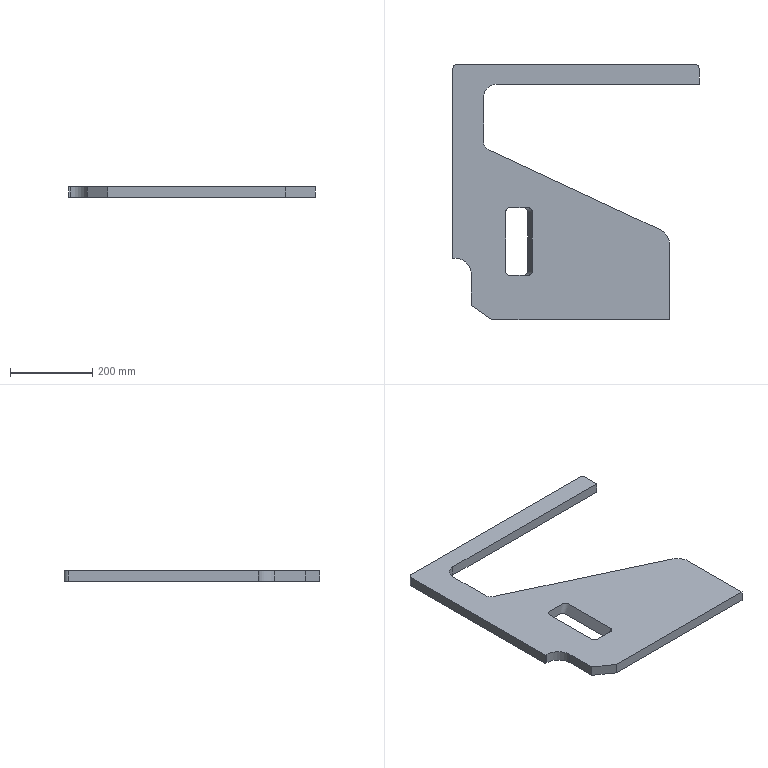Part | SolidWorks | features BlendCut 1, Extrusion 1 | 1 solid | 21 faces | box 600 x 622.5 x 25 mm | volume 4943914 mm3 | plane 13 | cylinder 6 | spline 2 | commonest cylinder face diameters 20 x2 80 x2 40 x1 60 x1
STEP:
#1=CARTESIAN_POINT('',(182.5,263.,0.));
#2=VERTEX_POINT('',#1);
#3=CARTESIAN_POINT('',(182.5,118.,0.));
#4=VERTEX_POINT('',#3);
#5=CARTESIAN_POINT('',(182.5,263.,0.));
#6=DIRECTION('',(0.,-1.,0.));
#7=VECTOR('',#6,1000.);
#8=LINE('',#5,#7);
#9=EDGE_CURVE('',#2,#4,#8,.T.);
#10=ORIENTED_EDGE('',*,*,#9,.T.);
#11=CARTESIAN_POINT('',(193.5,118.,25.));
#12=VERTEX_POINT('',#11);
#13=CARTESIAN_POINT('',(182.5,118.,0.));
#14=CARTESIAN_POINT('',(193.5,118.,25.));
#15=B_SPLINE_CURVE_WITH_KNOTS('',1,(#13,#14),.UNSPECIFIED.,.F.,.F.,(2,2),(0.,1.),.UNSPECIFIED.);
#16=EDGE_CURVE('',#4,#12,#15,.T.);
#17=ORIENTED_EDGE('',*,*,#16,.T.);
#18=CARTESIAN_POINT('',(193.5,263.,25.));
#19=VERTEX_POINT('',#18);
#20=CARTESIAN_POINT('',(193.5,263.,25.));
#21=DIRECTION('',(0.,1.,0.));
#22=VECTOR('',#21,1000.);
#23=LINE('',#20,#22);
#24=EDGE_CURVE('',#12,#19,#23,.T.);
#25=ORIENTED_EDGE('',*,*,#24,.T.);
#26=CARTESIAN_POINT('',(183.5,273.,25.));
#27=VERTEX_POINT('',#26);
#28=CARTESIAN_POINT('',(183.5,263.,25.));
#29=DIRECTION('',(0.,0.,1.));
#30=DIRECTION('',(-1.,0.,0.));
#31=AXIS2_PLACEMENT_3D('',#28,#29,#30);
#32=CIRCLE('',#31,10.);
#33=EDGE_CURVE('',#19,#27,#32,.T.);
#34=ORIENTED_EDGE('',*,*,#33,.T.);
#35=CARTESIAN_POINT('',(138.5,273.,25.));
#36=VERTEX_POINT('',#35);
#37=CARTESIAN_POINT('',(138.5,273.,25.));
#38=DIRECTION('',(-1.,0.,0.));
#39=VECTOR('',#38,1000.);
#40=LINE('',#37,#39);
#41=EDGE_CURVE('',#27,#36,#40,.T.);
#42=ORIENTED_EDGE('',*,*,#41,.T.);
#43=CARTESIAN_POINT('',(128.5,263.,25.));
#44=VERTEX_POINT('',#43);
#45=CARTESIAN_POINT('',(138.5,263.,25.));
#46=DIRECTION('',(0.,0.,1.));
#47=DIRECTION('',(-1.,0.,0.));
#48=AXIS2_PLACEMENT_3D('',#45,#46,#47);
#49=CIRCLE('',#48,10.);
#50=EDGE_CURVE('',#36,#44,#49,.T.);
#51=ORIENTED_EDGE('',*,*,#50,.T.);
#52=CARTESIAN_POINT('',(128.5,263.,0.));
#53=VERTEX_POINT('',#52);
#54=CARTESIAN_POINT('',(128.5,263.,0.));
#55=CARTESIAN_POINT('',(128.5,263.,25.));
#56=B_SPLINE_CURVE_WITH_KNOTS('',1,(#54,#55),.UNSPECIFIED.,.F.,.F.,(2,2),(0.,1.),.UNSPECIFIED.);
#57=EDGE_CURVE('',#53,#44,#56,.T.);
#58=ORIENTED_EDGE('',*,*,#57,.F.);
#59=CARTESIAN_POINT('',(138.5,273.,0.));
#60=VERTEX_POINT('',#59);
#61=CARTESIAN_POINT('',(138.5,263.,0.));
#62=DIRECTION('',(0.,0.,-1.));
#63=DIRECTION('',(-1.,0.,0.));
#64=AXIS2_PLACEMENT_3D('',#61,#62,#63);
#65=CIRCLE('',#64,10.);
#66=EDGE_CURVE('',#53,#60,#65,.T.);
#67=ORIENTED_EDGE('',*,*,#66,.T.);
#68=CARTESIAN_POINT('',(172.5,273.,0.));
#69=VERTEX_POINT('',#68);
#70=CARTESIAN_POINT('',(138.5,273.,0.));
#71=DIRECTION('',(1.,0.,0.));
#72=VECTOR('',#71,1000.);
#73=LINE('',#70,#72);
#74=EDGE_CURVE('',#60,#69,#73,.T.);
#75=ORIENTED_EDGE('',*,*,#74,.T.);
#76=CARTESIAN_POINT('',(172.5,263.,0.));
#77=DIRECTION('',(0.,0.,-1.));
#78=DIRECTION('',(1.,0.,0.));
#79=AXIS2_PLACEMENT_3D('',#76,#77,#78);
#80=CIRCLE('',#79,10.);
#81=EDGE_CURVE('',#69,#2,#80,.T.);
#82=ORIENTED_EDGE('',*,*,#81,.T.);
#83=EDGE_LOOP('',(#10,#17,#25,#34,#42,#51,#58,#67,#75,#82));
#84=FACE_OUTER_BOUND('',#83,.T.);
#85=CARTESIAN_POINT('',(128.5,263.,0.));
#86=CARTESIAN_POINT('',(128.5,263.,25.));
#87=CARTESIAN_POINT('',(128.5,250.917,0.));
#88=CARTESIAN_POINT('',(128.5,250.917,25.));
#89=CARTESIAN_POINT('',(128.5,226.75,0.));
#90=CARTESIAN_POINT('',(128.5,226.75,25.));
#91=CARTESIAN_POINT('',(128.5,190.5,0.));
#92=CARTESIAN_POINT('',(128.5,190.5,25.));
#93=CARTESIAN_POINT('',(128.5,154.25,0.));
#94=CARTESIAN_POINT('',(128.5,154.25,25.));
#95=CARTESIAN_POINT('',(128.5,130.083,0.));
#96=CARTESIAN_POINT('',(128.5,130.083,25.));
#97=CARTESIAN_POINT('',(128.5,116.691,0.));
#98=CARTESIAN_POINT('',(128.5,116.691,25.));
#99=CARTESIAN_POINT('',(129.027,113.997,0.));
#100=CARTESIAN_POINT('',(129.014,114.136,25.));
#101=CARTESIAN_POINT('',(131.408,110.559,0.));
#102=CARTESIAN_POINT('',(131.118,110.896,25.));
#103=CARTESIAN_POINT('',(134.844,108.424,0.));
#104=CARTESIAN_POINT('',(134.338,108.618,25.));
#105=CARTESIAN_POINT('',(137.318,108.,0.));
#106=CARTESIAN_POINT('',(137.057,108.,25.));
#107=CARTESIAN_POINT('',(141.461,108.,0.));
#108=CARTESIAN_POINT('',(142.116,108.,25.));
#109=CARTESIAN_POINT('',(147.179,108.,0.));
#110=CARTESIAN_POINT('',(149.538,108.,25.));
#111=CARTESIAN_POINT('',(155.5,108.,0.));
#112=CARTESIAN_POINT('',(161.,108.,25.));
#113=CARTESIAN_POINT('',(163.821,108.,0.));
#114=CARTESIAN_POINT('',(172.462,108.,25.));
#115=CARTESIAN_POINT('',(169.539,108.,0.));
#116=CARTESIAN_POINT('',(179.884,108.,25.));
#117=CARTESIAN_POINT('',(173.682,108.,0.));
#118=CARTESIAN_POINT('',(184.943,108.,25.));
#119=CARTESIAN_POINT('',(176.156,108.424,0.));
#120=CARTESIAN_POINT('',(187.662,108.618,25.));
#121=CARTESIAN_POINT('',(179.592,110.559,0.));
#122=CARTESIAN_POINT('',(190.882,110.896,25.));
#123=CARTESIAN_POINT('',(181.973,113.997,0.));
#124=CARTESIAN_POINT('',(192.986,114.136,25.));
#125=CARTESIAN_POINT('',(182.5,116.691,0.));
#126=CARTESIAN_POINT('',(193.5,116.691,25.));
#127=CARTESIAN_POINT('',(182.5,130.083,0.));
#128=CARTESIAN_POINT('',(193.5,130.083,25.));
#129=CARTESIAN_POINT('',(182.5,154.25,0.));
#130=CARTESIAN_POINT('',(193.5,154.25,25.));
#131=CARTESIAN_POINT('',(182.5,190.5,0.));
#132=CARTESIAN_POINT('',(193.5,190.5,25.));
#133=CARTESIAN_POINT('',(182.5,226.75,0.));
#134=CARTESIAN_POINT('',(193.5,226.75,25.));
#135=CARTESIAN_POINT('',(182.5,250.917,0.));
#136=CARTESIAN_POINT('',(193.5,250.917,25.));
#137=CARTESIAN_POINT('',(182.5,264.309,0.));
#138=CARTESIAN_POINT('',(193.5,264.309,25.));
#139=CARTESIAN_POINT('',(181.973,267.003,0.));
#140=CARTESIAN_POINT('',(192.986,266.864,25.));
#141=CARTESIAN_POINT('',(179.592,270.441,0.));
#142=CARTESIAN_POINT('',(190.882,270.104,25.));
#143=CARTESIAN_POINT('',(176.156,272.576,0.));
#144=CARTESIAN_POINT('',(187.662,272.382,25.));
#145=CARTESIAN_POINT('',(173.682,273.,0.));
#146=CARTESIAN_POINT('',(184.943,273.,25.));
#147=CARTESIAN_POINT('',(169.539,273.,0.));
#148=CARTESIAN_POINT('',(179.884,273.,25.));
#149=CARTESIAN_POINT('',(163.821,273.,0.));
#150=CARTESIAN_POINT('',(172.462,273.,25.));
#151=CARTESIAN_POINT('',(155.5,273.,0.));
#152=CARTESIAN_POINT('',(161.,273.,25.));
#153=CARTESIAN_POINT('',(147.179,273.,0.));
#154=CARTESIAN_POINT('',(149.538,273.,25.));
#155=CARTESIAN_POINT('',(141.461,273.,0.));
#156=CARTESIAN_POINT('',(142.116,273.,25.));
#157=CARTESIAN_POINT('',(137.318,273.,0.));
#158=CARTESIAN_POINT('',(137.057,273.,25.));
#159=CARTESIAN_POINT('',(134.844,272.576,0.));
#160=CARTESIAN_POINT('',(134.338,272.382,25.));
#161=CARTESIAN_POINT('',(131.408,270.441,0.));
#162=CARTESIAN_POINT('',(131.118,270.104,25.));
#163=CARTESIAN_POINT('',(129.027,267.003,0.));
#164=CARTESIAN_POINT('',(129.014,266.864,25.));
#165=CARTESIAN_POINT('',(128.5,264.309,0.));
#166=CARTESIAN_POINT('',(128.5,264.309,25.));
#167=CARTESIAN_POINT('',(128.5,263.,0.));
#168=CARTESIAN_POINT('',(128.5,263.,25.));
#169=B_SPLINE_SURFACE_WITH_KNOTS('',3,1,((#85,#86),(#87,#88),(#89,#90),(#91,#92),(#93,#94),(#95,#96),(#97,#98),(#99,#100),(#101,#102),(#103,#104),(#105,#106),(#107,#108),(#109,#110),(#111,#112),(#113,#114),(#115,#116),(#117,#118),(#119,#120),(#121,#122),(#123,#124),(#125,#126),(#127,#128),(#129,#130),(#131,#132),(#133,#134),(#135,#136),(#137,#138),(#139,#140),(#141,#142),(#143,#144),(#145,#146),(#147,#148),(#149,#150),(#151,#152),(#153,#154),(#155,#156),(#157,#158),(#159,#160),(#161,#162),(#163,#164),(#165,#166),(#167,#168)),.UNSPECIFIED.,.T.,.F.,.F.,(4,1,1,1,2,1,1,1,2,1,1,1,2,1,1,1,2,1,1,1,2,1,1,1,2,1,1,1,2,1,1,1,4),(2,2),(0.,0.084,0.168,0.252,0.336,0.3451,0.3542,0.3633,0.3724,0.3952,0.418,0.4408,0.4636,0.4727,0.4818,0.4909,0.5,0.584,0.668,0.752,0.836,0.8451,0.8542,0.8633,0.8724,0.8952,0.918,0.9408,0.9636,0.9727,0.9818,0.9909,1.),(0.,1.),.UNSPECIFIED.);
#170=ADVANCED_FACE('',(#84),#169,.F.);
#171=CARTESIAN_POINT('',(5.,150.,0.));
#172=VERTEX_POINT('',#171);
#173=CARTESIAN_POINT('',(45.,110.,0.));
#174=VERTEX_POINT('',#173);
#175=CARTESIAN_POINT('',(5.,110.,0.));
#176=DIRECTION('',(0.,0.,-1.));
#177=DIRECTION('',(-1.,0.,0.));
#178=AXIS2_PLACEMENT_3D('',#175,#176,#177);
#179=CIRCLE('',#178,40.);
#180=EDGE_CURVE('',#172,#174,#179,.T.);
#181=ORIENTED_EDGE('',*,*,#180,.T.);
#182=CARTESIAN_POINT('',(45.,110.,25.));
#183=VERTEX_POINT('',#182);
#184=CARTESIAN_POINT('',(45.,110.,25.));
#185=DIRECTION('',(0.,0.,-1.));
#186=VECTOR('',#185,1000.);
#187=LINE('',#184,#186);
#188=EDGE_CURVE('',#183,#174,#187,.T.);
#189=ORIENTED_EDGE('',*,*,#188,.F.);
#190=CARTESIAN_POINT('',(5.,150.,25.));
#191=VERTEX_POINT('',#190);
#192=CARTESIAN_POINT('',(5.,110.,25.));
#193=DIRECTION('',(0.,0.,-1.));
#194=DIRECTION('',(-1.,0.,0.));
#195=AXIS2_PLACEMENT_3D('',#192,#193,#194);
#196=CIRCLE('',#195,40.);
#197=EDGE_CURVE('',#191,#183,#196,.T.);
#198=ORIENTED_EDGE('',*,*,#197,.F.);
#199=CARTESIAN_POINT('',(5.,150.,25.));
#200=DIRECTION('',(0.,0.,-1.));
#201=VECTOR('',#200,1000.);
#202=LINE('',#199,#201);
#203=EDGE_CURVE('',#191,#172,#202,.T.);
#204=ORIENTED_EDGE('',*,*,#203,.T.);
#205=EDGE_LOOP('',(#181,#189,#198,#204));
#206=FACE_OUTER_BOUND('',#205,.T.);
#207=CARTESIAN_POINT('',(5.,110.,25.));
#208=DIRECTION('',(0.,0.,-1.));
#209=DIRECTION('',(-1.,0.,0.));
#210=AXIS2_PLACEMENT_3D('',#207,#208,#209);
#211=CYLINDRICAL_SURFACE('',#210,40.);
#212=ADVANCED_FACE('',(#206),#211,.F.);
#213=CARTESIAN_POINT('',(45.,35.01,0.));
#214=VERTEX_POINT('',#213);
#215=CARTESIAN_POINT('',(45.,35.01,0.));
#216=DIRECTION('',(0.,-1.,0.));
#217=VECTOR('',#216,1000.);
#218=LINE('',#215,#217);
#219=EDGE_CURVE('',#174,#214,#218,.T.);
#220=ORIENTED_EDGE('',*,*,#219,.T.);
#221=CARTESIAN_POINT('',(45.,35.01,25.));
#222=VERTEX_POINT('',#221);
#223=CARTESIAN_POINT('',(45.,35.01,25.));
#224=DIRECTION('',(0.,0.,-1.));
#225=VECTOR('',#224,1000.);
#226=LINE('',#223,#225);
#227=EDGE_CURVE('',#222,#214,#226,.T.);
#228=ORIENTED_EDGE('',*,*,#227,.F.);
#229=CARTESIAN_POINT('',(45.,35.01,25.));
#230=DIRECTION('',(0.,-1.,0.));
#231=VECTOR('',#230,1000.);
#232=LINE('',#229,#231);
#233=EDGE_CURVE('',#183,#222,#232,.T.);
#234=ORIENTED_EDGE('',*,*,#233,.F.);
#235=ORIENTED_EDGE('',*,*,#188,.T.);
#236=EDGE_LOOP('',(#220,#228,#234,#235));
#237=FACE_OUTER_BOUND('',#236,.T.);
#238=CARTESIAN_POINT('',(45.,35.01,25.));
#239=DIRECTION('',(1.,0.,0.));
#240=DIRECTION('',(0.,0.,-1.));
#241=AXIS2_PLACEMENT_3D('',#238,#239,#240);
#242=PLANE('',#241);
#243=ADVANCED_FACE('',(#237),#242,.F.);
#244=CARTESIAN_POINT('',(95.,0.,0.));
#245=VERTEX_POINT('',#244);
#246=CARTESIAN_POINT('',(95.,0.,0.));
#247=DIRECTION('',(0.8192,-0.5736,0.));
#248=VECTOR('',#247,1000.);
#249=LINE('',#246,#248);
#250=EDGE_CURVE('',#214,#245,#249,.T.);
#251=ORIENTED_EDGE('',*,*,#250,.T.);
#252=CARTESIAN_POINT('',(95.,0.,25.));
#253=VERTEX_POINT('',#252);
#254=CARTESIAN_POINT('',(95.,0.,25.));
#255=DIRECTION('',(0.,0.,-1.));
#256=VECTOR('',#255,1000.);
#257=LINE('',#254,#256);
#258=EDGE_CURVE('',#253,#245,#257,.T.);
#259=ORIENTED_EDGE('',*,*,#258,.F.);
#260=CARTESIAN_POINT('',(95.,0.,25.));
#261=DIRECTION('',(0.8192,-0.5736,0.));
#262=VECTOR('',#261,1000.);
#263=LINE('',#260,#262);
#264=EDGE_CURVE('',#222,#253,#263,.T.);
#265=ORIENTED_EDGE('',*,*,#264,.F.);
#266=ORIENTED_EDGE('',*,*,#227,.T.);
#267=EDGE_LOOP('',(#251,#259,#265,#266));
#268=FACE_OUTER_BOUND('',#267,.T.);
#269=CARTESIAN_POINT('',(95.,0.,25.));
#270=DIRECTION('',(0.5736,0.8192,0.));
#271=DIRECTION('',(-0.8192,0.5736,0.));
#272=AXIS2_PLACEMENT_3D('',#269,#270,#271);
#273=PLANE('',#272);
#274=ADVANCED_FACE('',(#268),#273,.F.);
#275=CARTESIAN_POINT('',(528.,0.,0.));
#276=VERTEX_POINT('',#275);
#277=CARTESIAN_POINT('',(528.,0.,0.));
#278=DIRECTION('',(1.,0.,0.));
#279=VECTOR('',#278,1000.);
#280=LINE('',#277,#279);
#281=EDGE_CURVE('',#245,#276,#280,.T.);
#282=ORIENTED_EDGE('',*,*,#281,.T.);
#283=CARTESIAN_POINT('',(528.,0.,25.));
#284=VERTEX_POINT('',#283);
#285=CARTESIAN_POINT('',(528.,0.,25.));
#286=DIRECTION('',(0.,0.,-1.));
#287=VECTOR('',#286,1000.);
#288=LINE('',#285,#287);
#289=EDGE_CURVE('',#284,#276,#288,.T.);
#290=ORIENTED_EDGE('',*,*,#289,.F.);
#291=CARTESIAN_POINT('',(528.,0.,25.));
#292=DIRECTION('',(1.,0.,0.));
#293=VECTOR('',#292,1000.);
#294=LINE('',#291,#293);
#295=EDGE_CURVE('',#253,#284,#294,.T.);
#296=ORIENTED_EDGE('',*,*,#295,.F.);
#297=ORIENTED_EDGE('',*,*,#258,.T.);
#298=EDGE_LOOP('',(#282,#290,#296,#297));
#299=FACE_OUTER_BOUND('',#298,.T.);
#300=CARTESIAN_POINT('',(528.,0.,25.));
#301=DIRECTION('',(0.,1.,0.));
#302=DIRECTION('',(-1.,0.,0.));
#303=AXIS2_PLACEMENT_3D('',#300,#301,#302);
#304=PLANE('',#303);
#305=ADVANCED_FACE('',(#299),#304,.F.);
#306=CARTESIAN_POINT('',(528.,183.025,0.));
#307=VERTEX_POINT('',#306);
#308=CARTESIAN_POINT('',(528.,183.025,0.));
#309=DIRECTION('',(0.,1.,0.));
#310=VECTOR('',#309,1000.);
#311=LINE('',#308,#310);
#312=EDGE_CURVE('',#276,#307,#311,.T.);
#313=ORIENTED_EDGE('',*,*,#312,.T.);
#314=CARTESIAN_POINT('',(528.,183.025,25.));
#315=VERTEX_POINT('',#314);
#316=CARTESIAN_POINT('',(528.,183.025,25.));
#317=DIRECTION('',(0.,0.,-1.));
#318=VECTOR('',#317,1000.);
#319=LINE('',#316,#318);
#320=EDGE_CURVE('',#315,#307,#319,.T.);
#321=ORIENTED_EDGE('',*,*,#320,.F.);
#322=CARTESIAN_POINT('',(528.,183.025,25.));
#323=DIRECTION('',(0.,1.,0.));
#324=VECTOR('',#323,1000.);
#325=LINE('',#322,#324);
#326=EDGE_CURVE('',#284,#315,#325,.T.);
#327=ORIENTED_EDGE('',*,*,#326,.F.);
#328=ORIENTED_EDGE('',*,*,#289,.T.);
#329=EDGE_LOOP('',(#313,#321,#327,#328));
#330=FACE_OUTER_BOUND('',#329,.T.);
#331=CARTESIAN_POINT('',(528.,183.025,25.));
#332=DIRECTION('',(-1.,0.,0.));
#333=DIRECTION('',(0.,0.,1.));
#334=AXIS2_PLACEMENT_3D('',#331,#332,#333);
#335=PLANE('',#334);
#336=ADVANCED_FACE('',(#330),#335,.F.);
#337=CARTESIAN_POINT('',(504.915,219.273,0.));
#338=VERTEX_POINT('',#337);
#339=CARTESIAN_POINT('',(488.,183.025,0.));
#340=DIRECTION('',(0.,0.,1.));
#341=DIRECTION('',(1.,0.,0.));
#342=AXIS2_PLACEMENT_3D('',#339,#340,#341);
#343=CIRCLE('',#342,40.);
#344=EDGE_CURVE('',#307,#338,#343,.T.);
#345=ORIENTED_EDGE('',*,*,#344,.T.);
#346=CARTESIAN_POINT('',(504.915,219.273,25.));
#347=VERTEX_POINT('',#346);
#348=CARTESIAN_POINT('',(504.915,219.273,25.));
#349=DIRECTION('',(0.,0.,-1.));
#350=VECTOR('',#349,1000.);
#351=LINE('',#348,#350);
#352=EDGE_CURVE('',#347,#338,#351,.T.);
#353=ORIENTED_EDGE('',*,*,#352,.F.);
#354=CARTESIAN_POINT('',(488.,183.025,25.));
#355=DIRECTION('',(0.,0.,1.));
#356=DIRECTION('',(1.,0.,0.));
#357=AXIS2_PLACEMENT_3D('',#354,#355,#356);
#358=CIRCLE('',#357,40.);
#359=EDGE_CURVE('',#315,#347,#358,.T.);
#360=ORIENTED_EDGE('',*,*,#359,.F.);
#361=ORIENTED_EDGE('',*,*,#320,.T.);
#362=EDGE_LOOP('',(#345,#353,#360,#361));
#363=FACE_OUTER_BOUND('',#362,.T.);
#364=CARTESIAN_POINT('',(488.,183.025,25.));
#365=DIRECTION('',(0.,0.,-1.));
#366=DIRECTION('',(-1.,0.,0.));
#367=AXIS2_PLACEMENT_3D('',#364,#365,#366);
#368=CYLINDRICAL_SURFACE('',#367,40.);
#369=ADVANCED_FACE('',(#363),#368,.T.);
#370=CARTESIAN_POINT('',(86.542,414.514,0.));
#371=VERTEX_POINT('',#370);
#372=CARTESIAN_POINT('',(86.542,414.514,0.));
#373=DIRECTION('',(-0.9062,0.4229,0.));
#374=VECTOR('',#373,1000.);
#375=LINE('',#372,#374);
#376=EDGE_CURVE('',#338,#371,#375,.T.);
#377=ORIENTED_EDGE('',*,*,#376,.T.);
#378=CARTESIAN_POINT('',(86.542,414.514,25.));
#379=VERTEX_POINT('',#378);
#380=CARTESIAN_POINT('',(86.542,414.514,25.));
#381=DIRECTION('',(0.,0.,-1.));
#382=VECTOR('',#381,1000.);
#383=LINE('',#380,#382);
#384=EDGE_CURVE('',#379,#371,#383,.T.);
#385=ORIENTED_EDGE('',*,*,#384,.F.);
#386=CARTESIAN_POINT('',(86.542,414.514,25.));
#387=DIRECTION('',(-0.9062,0.4229,0.));
#388=VECTOR('',#387,1000.);
#389=LINE('',#386,#388);
#390=EDGE_CURVE('',#347,#379,#389,.T.);
#391=ORIENTED_EDGE('',*,*,#390,.F.);
#392=ORIENTED_EDGE('',*,*,#352,.T.);
#393=EDGE_LOOP('',(#377,#385,#391,#392));
#394=FACE_OUTER_BOUND('',#393,.T.);
#395=CARTESIAN_POINT('',(86.542,414.514,25.));
#396=DIRECTION('',(-0.4229,-0.9062,0.));
#397=DIRECTION('',(0.9062,-0.4229,0.));
#398=AXIS2_PLACEMENT_3D('',#395,#396,#397);
#399=PLANE('',#398);
#400=ADVANCED_FACE('',(#394),#399,.F.);
#401=CARTESIAN_POINT('',(75.,432.637,0.));
#402=VERTEX_POINT('',#401);
#403=CARTESIAN_POINT('',(95.,432.637,0.));
#404=DIRECTION('',(0.,0.,-1.));
#405=DIRECTION('',(1.,0.,0.));
#406=AXIS2_PLACEMENT_3D('',#403,#404,#405);
#407=CIRCLE('',#406,20.);
#408=EDGE_CURVE('',#371,#402,#407,.T.);
#409=ORIENTED_EDGE('',*,*,#408,.T.);
#410=CARTESIAN_POINT('',(75.,432.637,25.));
#411=VERTEX_POINT('',#410);
#412=CARTESIAN_POINT('',(75.,432.637,25.));
#413=DIRECTION('',(0.,0.,-1.));
#414=VECTOR('',#413,1000.);
#415=LINE('',#412,#414);
#416=EDGE_CURVE('',#411,#402,#415,.T.);
#417=ORIENTED_EDGE('',*,*,#416,.F.);
#418=CARTESIAN_POINT('',(95.,432.637,25.));
#419=DIRECTION('',(0.,0.,-1.));
#420=DIRECTION('',(1.,0.,0.));
#421=AXIS2_PLACEMENT_3D('',#418,#419,#420);
#422=CIRCLE('',#421,20.);
#423=EDGE_CURVE('',#379,#411,#422,.T.);
#424=ORIENTED_EDGE('',*,*,#423,.F.);
#425=ORIENTED_EDGE('',*,*,#384,.T.);
#426=EDGE_LOOP('',(#409,#417,#424,#425));
#427=FACE_OUTER_BOUND('',#426,.T.);
#428=CARTESIAN_POINT('',(95.,432.637,25.));
#429=DIRECTION('',(0.,0.,-1.));
#430=DIRECTION('',(-1.,0.,0.));
#431=AXIS2_PLACEMENT_3D('',#428,#429,#430);
#432=CYLINDRICAL_SURFACE('',#431,20.);
#433=ADVANCED_FACE('',(#427),#432,.F.);
#434=CARTESIAN_POINT('',(75.,543.5,0.));
#435=VERTEX_POINT('',#434);
#436=CARTESIAN_POINT('',(75.,543.5,0.));
#437=DIRECTION('',(0.,1.,0.));
#438=VECTOR('',#437,1000.);
#439=LINE('',#436,#438);
#440=EDGE_CURVE('',#402,#435,#439,.T.);
#441=ORIENTED_EDGE('',*,*,#440,.T.);
#442=CARTESIAN_POINT('',(75.,543.5,25.));
#443=VERTEX_POINT('',#442);
#444=CARTESIAN_POINT('',(75.,543.5,25.));
#445=DIRECTION('',(0.,0.,-1.));
#446=VECTOR('',#445,1000.);
#447=LINE('',#444,#446);
#448=EDGE_CURVE('',#443,#435,#447,.T.);
#449=ORIENTED_EDGE('',*,*,#448,.F.);
#450=CARTESIAN_POINT('',(75.,543.5,25.));
#451=DIRECTION('',(0.,1.,0.));
#452=VECTOR('',#451,1000.);
#453=LINE('',#450,#452);
#454=EDGE_CURVE('',#411,#443,#453,.T.);
#455=ORIENTED_EDGE('',*,*,#454,.F.);
#456=ORIENTED_EDGE('',*,*,#416,.T.);
#457=EDGE_LOOP('',(#441,#449,#455,#456));
#458=FACE_OUTER_BOUND('',#457,.T.);
#459=CARTESIAN_POINT('',(75.,543.5,25.));
#460=DIRECTION('',(-1.,0.,0.));
#461=DIRECTION('',(0.,-1.,0.));
#462=AXIS2_PLACEMENT_3D('',#459,#460,#461);
#463=PLANE('',#462);
#464=ADVANCED_FACE('',(#458),#463,.F.);
#465=CARTESIAN_POINT('',(105.,573.5,0.));
#466=VERTEX_POINT('',#465);
#467=CARTESIAN_POINT('',(105.,543.5,0.));
#468=DIRECTION('',(0.,0.,-1.));
#469=DIRECTION('',(-1.,0.,0.));
#470=AXIS2_PLACEMENT_3D('',#467,#468,#469);
#471=CIRCLE('',#470,30.);
#472=EDGE_CURVE('',#435,#466,#471,.T.);
#473=ORIENTED_EDGE('',*,*,#472,.T.);
#474=CARTESIAN_POINT('',(105.,573.5,25.));
#475=VERTEX_POINT('',#474);
#476=CARTESIAN_POINT('',(105.,573.5,25.));
#477=DIRECTION('',(0.,0.,-1.));
#478=VECTOR('',#477,1000.);
#479=LINE('',#476,#478);
#480=EDGE_CURVE('',#475,#466,#479,.T.);
#481=ORIENTED_EDGE('',*,*,#480,.F.);
#482=CARTESIAN_POINT('',(105.,543.5,25.));
#483=DIRECTION('',(0.,0.,-1.));
#484=DIRECTION('',(-1.,0.,0.));
#485=AXIS2_PLACEMENT_3D('',#482,#483,#484);
#486=CIRCLE('',#485,30.);
#487=EDGE_CURVE('',#443,#475,#486,.T.);
#488=ORIENTED_EDGE('',*,*,#487,.F.);
#489=ORIENTED_EDGE('',*,*,#448,.T.);
#490=EDGE_LOOP('',(#473,#481,#488,#489));
#491=FACE_OUTER_BOUND('',#490,.T.);
#492=CARTESIAN_POINT('',(105.,543.5,25.));
#493=DIRECTION('',(0.,0.,-1.));
#494=DIRECTION('',(-1.,0.,0.));
#495=AXIS2_PLACEMENT_3D('',#492,#493,#494);
#496=CYLINDRICAL_SURFACE('',#495,30.);
#497=ADVANCED_FACE('',(#491),#496,.F.);
#498=CARTESIAN_POINT('',(600.,573.5,0.));
#499=VERTEX_POINT('',#498);
#500=CARTESIAN_POINT('',(600.,573.5,0.));
#501=DIRECTION('',(1.,0.,0.));
#502=VECTOR('',#501,1000.);
#503=LINE('',#500,#502);
#504=EDGE_CURVE('',#466,#499,#503,.T.);
#505=ORIENTED_EDGE('',*,*,#504,.T.);
#506=CARTESIAN_POINT('',(600.,573.5,25.));
#507=VERTEX_POINT('',#506);
#508=CARTESIAN_POINT('',(600.,573.5,25.));
#509=DIRECTION('',(0.,0.,-1.));
#510=VECTOR('',#509,1000.);
#511=LINE('',#508,#510);
#512=EDGE_CURVE('',#507,#499,#511,.T.);
#513=ORIENTED_EDGE('',*,*,#512,.F.);
#514=CARTESIAN_POINT('',(600.,573.5,25.));
#515=DIRECTION('',(1.,0.,0.));
#516=VECTOR('',#515,1000.);
#517=LINE('',#514,#516);
#518=EDGE_CURVE('',#475,#507,#517,.T.);
#519=ORIENTED_EDGE('',*,*,#518,.F.);
#520=ORIENTED_EDGE('',*,*,#480,.T.);
#521=EDGE_LOOP('',(#505,#513,#519,#520));
#522=FACE_OUTER_BOUND('',#521,.T.);
#523=CARTESIAN_POINT('',(600.,573.5,25.));
#524=DIRECTION('',(0.,1.,0.));
#525=DIRECTION('',(-1.,0.,0.));
#526=AXIS2_PLACEMENT_3D('',#523,#524,#525);
#527=PLANE('',#526);
#528=ADVANCED_FACE('',(#522),#527,.F.);
#529=CARTESIAN_POINT('',(600.,612.5,0.));
#530=VERTEX_POINT('',#529);
#531=CARTESIAN_POINT('',(600.,612.5,0.));
#532=DIRECTION('',(0.,1.,0.));
#533=VECTOR('',#532,1000.);
#534=LINE('',#531,#533);
#535=EDGE_CURVE('',#499,#530,#534,.T.);
#536=ORIENTED_EDGE('',*,*,#535,.T.);
#537=CARTESIAN_POINT('',(600.,612.5,25.));
#538=VERTEX_POINT('',#537);
#539=CARTESIAN_POINT('',(600.,612.5,25.));
#540=DIRECTION('',(0.,0.,-1.));
#541=VECTOR('',#540,1000.);
#542=LINE('',#539,#541);
#543=EDGE_CURVE('',#538,#530,#542,.T.);
#544=ORIENTED_EDGE('',*,*,#543,.F.);
#545=CARTESIAN_POINT('',(600.,612.5,25.));
#546=DIRECTION('',(0.,1.,0.));
#547=VECTOR('',#546,1000.);
#548=LINE('',#545,#547);
#549=EDGE_CURVE('',#507,#538,#548,.T.);
#550=ORIENTED_EDGE('',*,*,#549,.F.);
#551=ORIENTED_EDGE('',*,*,#512,.T.);
#552=EDGE_LOOP('',(#536,#544,#550,#551));
#553=FACE_OUTER_BOUND('',#552,.T.);
#554=CARTESIAN_POINT('',(600.,612.5,25.));
#555=DIRECTION('',(-1.,0.,0.));
#556=DIRECTION('',(0.,0.,1.));
#557=AXIS2_PLACEMENT_3D('',#554,#555,#556);
#558=PLANE('',#557);
#559=ADVANCED_FACE('',(#553),#558,.F.);
#560=CARTESIAN_POINT('',(590.,622.5,0.));
#561=VERTEX_POINT('',#560);
#562=CARTESIAN_POINT('',(590.,612.5,0.));
#563=DIRECTION('',(0.,0.,1.));
#564=DIRECTION('',(-1.,0.,0.));
#565=AXIS2_PLACEMENT_3D('',#562,#563,#564);
#566=CIRCLE('',#565,10.);
#567=EDGE_CURVE('',#530,#561,#566,.T.);
#568=ORIENTED_EDGE('',*,*,#567,.T.);
#569=CARTESIAN_POINT('',(590.,622.5,25.));
#570=VERTEX_POINT('',#569);
#571=CARTESIAN_POINT('',(590.,622.5,25.));
#572=DIRECTION('',(0.,0.,-1.));
#573=VECTOR('',#572,1000.);
#574=LINE('',#571,#573);
#575=EDGE_CURVE('',#570,#561,#574,.T.);
#576=ORIENTED_EDGE('',*,*,#575,.F.);
#577=CARTESIAN_POINT('',(590.,612.5,25.));
#578=DIRECTION('',(0.,0.,1.));
#579=DIRECTION('',(-1.,0.,0.));
#580=AXIS2_PLACEMENT_3D('',#577,#578,#579);
#581=CIRCLE('',#580,10.);
#582=EDGE_CURVE('',#538,#570,#581,.T.);
#583=ORIENTED_EDGE('',*,*,#582,.F.);
#584=ORIENTED_EDGE('',*,*,#543,.T.);
#585=EDGE_LOOP('',(#568,#576,#583,#584));
#586=FACE_OUTER_BOUND('',#585,.T.);
#587=CARTESIAN_POINT('',(590.,612.5,25.));
#588=DIRECTION('',(0.,0.,-1.));
#589=DIRECTION('',(-1.,0.,0.));
#590=AXIS2_PLACEMENT_3D('',#587,#588,#589);
#591=CYLINDRICAL_SURFACE('',#590,10.);
#592=ADVANCED_FACE('',(#586),#591,.T.);
#593=CARTESIAN_POINT('',(10.,622.5,0.));
#594=VERTEX_POINT('',#593);
#595=CARTESIAN_POINT('',(10.,622.5,0.));
#596=DIRECTION('',(-1.,0.,0.));
#597=VECTOR('',#596,1000.);
#598=LINE('',#595,#597);
#599=EDGE_CURVE('',#561,#594,#598,.T.);
#600=ORIENTED_EDGE('',*,*,#599,.T.);
#601=CARTESIAN_POINT('',(10.,622.5,25.));
#602=VERTEX_POINT('',#601);
#603=CARTESIAN_POINT('',(10.,622.5,25.));
#604=DIRECTION('',(0.,0.,-1.));
#605=VECTOR('',#604,1000.);
#606=LINE('',#603,#605);
#607=EDGE_CURVE('',#602,#594,#606,.T.);
#608=ORIENTED_EDGE('',*,*,#607,.F.);
#609=CARTESIAN_POINT('',(10.,622.5,25.));
#610=DIRECTION('',(-1.,0.,0.));
#611=VECTOR('',#610,1000.);
#612=LINE('',#609,#611);
#613=EDGE_CURVE('',#570,#602,#612,.T.);
#614=ORIENTED_EDGE('',*,*,#613,.F.);
#615=ORIENTED_EDGE('',*,*,#575,.T.);
#616=EDGE_LOOP('',(#600,#608,#614,#615));
#617=FACE_OUTER_BOUND('',#616,.T.);
#618=CARTESIAN_POINT('',(10.,622.5,25.));
#619=DIRECTION('',(0.,-1.,0.));
#620=DIRECTION('',(0.,0.,-1.));
#621=AXIS2_PLACEMENT_3D('',#618,#619,#620);
#622=PLANE('',#621);
#623=ADVANCED_FACE('',(#617),#622,.F.);
#624=CARTESIAN_POINT('',(0.,612.5,0.));
#625=VERTEX_POINT('',#624);
#626=CARTESIAN_POINT('',(10.,612.5,0.));
#627=DIRECTION('',(0.,0.,1.));
#628=DIRECTION('',(-1.,0.,0.));
#629=AXIS2_PLACEMENT_3D('',#626,#627,#628);
#630=CIRCLE('',#629,10.);
#631=EDGE_CURVE('',#594,#625,#630,.T.);
#632=ORIENTED_EDGE('',*,*,#631,.T.);
#633=CARTESIAN_POINT('',(0.,612.5,25.));
#634=VERTEX_POINT('',#633);
#635=CARTESIAN_POINT('',(0.,612.5,25.));
#636=DIRECTION('',(0.,0.,-1.));
#637=VECTOR('',#636,1000.);
#638=LINE('',#635,#637);
#639=EDGE_CURVE('',#634,#625,#638,.T.);
#640=ORIENTED_EDGE('',*,*,#639,.F.);
#641=CARTESIAN_POINT('',(10.,612.5,25.));
#642=DIRECTION('',(0.,0.,1.));
#643=DIRECTION('',(-1.,0.,0.));
#644=AXIS2_PLACEMENT_3D('',#641,#642,#643);
#645=CIRCLE('',#644,10.);
#646=EDGE_CURVE('',#602,#634,#645,.T.);
#647=ORIENTED_EDGE('',*,*,#646,.F.);
#648=ORIENTED_EDGE('',*,*,#607,.T.);
#649=EDGE_LOOP('',(#632,#640,#647,#648));
#650=FACE_OUTER_BOUND('',#649,.T.);
#651=CARTESIAN_POINT('',(10.,612.5,25.));
#652=DIRECTION('',(0.,0.,-1.));
#653=DIRECTION('',(-1.,0.,0.));
#654=AXIS2_PLACEMENT_3D('',#651,#652,#653);
#655=CYLINDRICAL_SURFACE('',#654,10.);
#656=ADVANCED_FACE('',(#650),#655,.T.);
#657=CARTESIAN_POINT('',(0.,150.,0.));
#658=VERTEX_POINT('',#657);
#659=CARTESIAN_POINT('',(0.,150.,0.));
#660=DIRECTION('',(0.,-1.,0.));
#661=VECTOR('',#660,1000.);
#662=LINE('',#659,#661);
#663=EDGE_CURVE('',#625,#658,#662,.T.);
#664=ORIENTED_EDGE('',*,*,#663,.T.);
#665=CARTESIAN_POINT('',(0.,150.,25.));
#666=VERTEX_POINT('',#665);
#667=CARTESIAN_POINT('',(0.,150.,25.));
#668=DIRECTION('',(0.,0.,-1.));
#669=VECTOR('',#668,1000.);
#670=LINE('',#667,#669);
#671=EDGE_CURVE('',#666,#658,#670,.T.);
#672=ORIENTED_EDGE('',*,*,#671,.F.);
#673=CARTESIAN_POINT('',(0.,150.,25.));
#674=DIRECTION('',(0.,-1.,0.));
#675=VECTOR('',#674,1000.);
#676=LINE('',#673,#675);
#677=EDGE_CURVE('',#634,#666,#676,.T.);
#678=ORIENTED_EDGE('',*,*,#677,.F.);
#679=ORIENTED_EDGE('',*,*,#639,.T.);
#680=EDGE_LOOP('',(#664,#672,#678,#679));
#681=FACE_OUTER_BOUND('',#680,.T.);
#682=CARTESIAN_POINT('',(0.,150.,25.));
#683=DIRECTION('',(1.,0.,0.));
#684=DIRECTION('',(0.,0.,-1.));
#685=AXIS2_PLACEMENT_3D('',#682,#683,#684);
#686=PLANE('',#685);
#687=ADVANCED_FACE('',(#681),#686,.F.);
#688=CARTESIAN_POINT('',(5.,150.,0.));
#689=DIRECTION('',(1.,0.,0.));
#690=VECTOR('',#689,1000.);
#691=LINE('',#688,#690);
#692=EDGE_CURVE('',#658,#172,#691,.T.);
#693=ORIENTED_EDGE('',*,*,#692,.T.);
#694=ORIENTED_EDGE('',*,*,#203,.F.);
#695=CARTESIAN_POINT('',(5.,150.,25.));
#696=DIRECTION('',(1.,0.,0.));
#697=VECTOR('',#696,1000.);
#698=LINE('',#695,#697);
#699=EDGE_CURVE('',#666,#191,#698,.T.);
#700=ORIENTED_EDGE('',*,*,#699,.F.);
#701=ORIENTED_EDGE('',*,*,#671,.T.);
#702=EDGE_LOOP('',(#693,#694,#700,#701));
#703=FACE_OUTER_BOUND('',#702,.T.);
#704=CARTESIAN_POINT('',(5.,150.,25.));
#705=DIRECTION('',(0.,1.,0.));
#706=DIRECTION('',(0.,0.,1.));
#707=AXIS2_PLACEMENT_3D('',#704,#705,#706);
#708=PLANE('',#707);
#709=ADVANCED_FACE('',(#703),#708,.F.);
#710=CARTESIAN_POINT('',(128.5,118.,25.));
#711=VERTEX_POINT('',#710);
#712=CARTESIAN_POINT('',(128.5,263.,25.));
#713=DIRECTION('',(0.,-1.,0.));
#714=VECTOR('',#713,1000.);
#715=LINE('',#712,#714);
#716=EDGE_CURVE('',#44,#711,#715,.T.);
#717=ORIENTED_EDGE('',*,*,#716,.F.);
#718=ORIENTED_EDGE('',*,*,#50,.F.);
#719=ORIENTED_EDGE('',*,*,#41,.F.);
#720=ORIENTED_EDGE('',*,*,#33,.F.);
#721=ORIENTED_EDGE('',*,*,#24,.F.);
#722=CARTESIAN_POINT('',(183.5,108.,25.));
#723=VERTEX_POINT('',#722);
#724=CARTESIAN_POINT('',(183.5,118.,25.));
#725=DIRECTION('',(0.,0.,1.));
#726=DIRECTION('',(-1.,0.,0.));
#727=AXIS2_PLACEMENT_3D('',#724,#725,#726);
#728=CIRCLE('',#727,10.);
#729=EDGE_CURVE('',#723,#12,#728,.T.);
#730=ORIENTED_EDGE('',*,*,#729,.F.);
#731=CARTESIAN_POINT('',(138.5,108.,25.));
#732=VERTEX_POINT('',#731);
#733=CARTESIAN_POINT('',(138.5,108.,25.));
#734=DIRECTION('',(1.,0.,0.));
#735=VECTOR('',#734,1000.);
#736=LINE('',#733,#735);
#737=EDGE_CURVE('',#732,#723,#736,.T.);
#738=ORIENTED_EDGE('',*,*,#737,.F.);
#739=CARTESIAN_POINT('',(138.5,118.,25.));
#740=DIRECTION('',(0.,0.,1.));
#741=DIRECTION('',(1.,0.,0.));
#742=AXIS2_PLACEMENT_3D('',#739,#740,#741);
#743=CIRCLE('',#742,10.);
#744=EDGE_CURVE('',#711,#732,#743,.T.);
#745=ORIENTED_EDGE('',*,*,#744,.F.);
#746=EDGE_LOOP('',(#717,#718,#719,#720,#721,#730,#738,#745));
#747=FACE_BOUND('',#746,.T.);
#748=ORIENTED_EDGE('',*,*,#197,.T.);
#749=ORIENTED_EDGE('',*,*,#233,.T.);
#750=ORIENTED_EDGE('',*,*,#264,.T.);
#751=ORIENTED_EDGE('',*,*,#295,.T.);
#752=ORIENTED_EDGE('',*,*,#326,.T.);
#753=ORIENTED_EDGE('',*,*,#359,.T.);
#754=ORIENTED_EDGE('',*,*,#390,.T.);
#755=ORIENTED_EDGE('',*,*,#423,.T.);
#756=ORIENTED_EDGE('',*,*,#454,.T.);
#757=ORIENTED_EDGE('',*,*,#487,.T.);
#758=ORIENTED_EDGE('',*,*,#518,.T.);
#759=ORIENTED_EDGE('',*,*,#549,.T.);
#760=ORIENTED_EDGE('',*,*,#582,.T.);
#761=ORIENTED_EDGE('',*,*,#613,.T.);
#762=ORIENTED_EDGE('',*,*,#646,.T.);
#763=ORIENTED_EDGE('',*,*,#677,.T.);
#764=ORIENTED_EDGE('',*,*,#699,.T.);
#765=EDGE_LOOP('',(#748,#749,#750,#751,#752,#753,#754,#755,#756,#757,#758,#759,#760,#761,#762,#763,#764));
#766=FACE_OUTER_BOUND('',#765,.T.);
#767=CARTESIAN_POINT('',(5.,110.,25.));
#768=DIRECTION('',(0.,0.,-1.));
#769=DIRECTION('',(-1.,0.,0.));
#770=AXIS2_PLACEMENT_3D('',#767,#768,#769);
#771=PLANE('',#770);
#772=ADVANCED_FACE('',(#747,#766),#771,.F.);
#773=ORIENTED_EDGE('',*,*,#66,.F.);
#774=CARTESIAN_POINT('',(128.5,118.,0.));
#775=VERTEX_POINT('',#774);
#776=CARTESIAN_POINT('',(128.5,263.,0.));
#777=DIRECTION('',(0.,1.,0.));
#778=VECTOR('',#777,1000.);
#779=LINE('',#776,#778);
#780=EDGE_CURVE('',#775,#53,#779,.T.);
#781=ORIENTED_EDGE('',*,*,#780,.F.);
#782=CARTESIAN_POINT('',(138.5,108.,0.));
#783=VERTEX_POINT('',#782);
#784=CARTESIAN_POINT('',(138.5,118.,0.));
#785=DIRECTION('',(0.,0.,-1.));
#786=DIRECTION('',(-1.,0.,0.));
#787=AXIS2_PLACEMENT_3D('',#784,#785,#786);
#788=CIRCLE('',#787,10.);
#789=EDGE_CURVE('',#783,#775,#788,.T.);
#790=ORIENTED_EDGE('',*,*,#789,.F.);
#791=CARTESIAN_POINT('',(172.5,108.,0.));
#792=VERTEX_POINT('',#791);
#793=CARTESIAN_POINT('',(138.5,108.,0.));
#794=DIRECTION('',(-1.,0.,0.));
#795=VECTOR('',#794,1000.);
#796=LINE('',#793,#795);
#797=EDGE_CURVE('',#792,#783,#796,.T.);
#798=ORIENTED_EDGE('',*,*,#797,.F.);
#799=CARTESIAN_POINT('',(172.5,118.,0.));
#800=DIRECTION('',(0.,0.,-1.));
#801=DIRECTION('',(1.,0.,0.));
#802=AXIS2_PLACEMENT_3D('',#799,#800,#801);
#803=CIRCLE('',#802,10.);
#804=EDGE_CURVE('',#4,#792,#803,.T.);
#805=ORIENTED_EDGE('',*,*,#804,.F.);
#806=ORIENTED_EDGE('',*,*,#9,.F.);
#807=ORIENTED_EDGE('',*,*,#81,.F.);
#808=ORIENTED_EDGE('',*,*,#74,.F.);
#809=EDGE_LOOP('',(#773,#781,#790,#798,#805,#806,#807,#808));
#810=FACE_BOUND('',#809,.T.);
#811=ORIENTED_EDGE('',*,*,#180,.F.);
#812=ORIENTED_EDGE('',*,*,#692,.F.);
#813=ORIENTED_EDGE('',*,*,#663,.F.);
#814=ORIENTED_EDGE('',*,*,#631,.F.);
#815=ORIENTED_EDGE('',*,*,#599,.F.);
#816=ORIENTED_EDGE('',*,*,#567,.F.);
#817=ORIENTED_EDGE('',*,*,#535,.F.);
#818=ORIENTED_EDGE('',*,*,#504,.F.);
#819=ORIENTED_EDGE('',*,*,#472,.F.);
#820=ORIENTED_EDGE('',*,*,#440,.F.);
#821=ORIENTED_EDGE('',*,*,#408,.F.);
#822=ORIENTED_EDGE('',*,*,#376,.F.);
#823=ORIENTED_EDGE('',*,*,#344,.F.);
#824=ORIENTED_EDGE('',*,*,#312,.F.);
#825=ORIENTED_EDGE('',*,*,#281,.F.);
#826=ORIENTED_EDGE('',*,*,#250,.F.);
#827=ORIENTED_EDGE('',*,*,#219,.F.);
#828=EDGE_LOOP('',(#811,#812,#813,#814,#815,#816,#817,#818,#819,#820,#821,#822,#823,#824,#825,#826,#827));
#829=FACE_OUTER_BOUND('',#828,.T.);
#830=CARTESIAN_POINT('',(5.,110.,0.));
#831=DIRECTION('',(0.,0.,-1.));
#832=DIRECTION('',(-1.,0.,0.));
#833=AXIS2_PLACEMENT_3D('',#830,#831,#832);
#834=PLANE('',#833);
#835=ADVANCED_FACE('',(#810,#829),#834,.T.);
#836=ORIENTED_EDGE('',*,*,#16,.F.);
#837=ORIENTED_EDGE('',*,*,#804,.T.);
#838=ORIENTED_EDGE('',*,*,#797,.T.);
#839=ORIENTED_EDGE('',*,*,#789,.T.);
#840=ORIENTED_EDGE('',*,*,#780,.T.);
#841=ORIENTED_EDGE('',*,*,#57,.T.);
#842=ORIENTED_EDGE('',*,*,#716,.T.);
#843=ORIENTED_EDGE('',*,*,#744,.T.);
#844=ORIENTED_EDGE('',*,*,#737,.T.);
#845=ORIENTED_EDGE('',*,*,#729,.T.);
#846=EDGE_LOOP('',(#836,#837,#838,#839,#840,#841,#842,#843,#844,#845));
#847=FACE_OUTER_BOUND('',#846,.T.);
#848=CARTESIAN_POINT('',(128.5,263.,0.));
#849=CARTESIAN_POINT('',(128.5,263.,25.));
#850=CARTESIAN_POINT('',(128.5,250.917,0.));
#851=CARTESIAN_POINT('',(128.5,250.917,25.));
#852=CARTESIAN_POINT('',(128.5,226.75,0.));
#853=CARTESIAN_POINT('',(128.5,226.75,25.));
#854=CARTESIAN_POINT('',(128.5,190.5,0.));
#855=CARTESIAN_POINT('',(128.5,190.5,25.));
#856=CARTESIAN_POINT('',(128.5,154.25,0.));
#857=CARTESIAN_POINT('',(128.5,154.25,25.));
#858=CARTESIAN_POINT('',(128.5,130.083,0.));
#859=CARTESIAN_POINT('',(128.5,130.083,25.));
#860=CARTESIAN_POINT('',(128.5,116.691,0.));
#861=CARTESIAN_POINT('',(128.5,116.691,25.));
#862=CARTESIAN_POINT('',(129.027,113.997,0.));
#863=CARTESIAN_POINT('',(129.014,114.136,25.));
#864=CARTESIAN_POINT('',(131.408,110.559,0.));
#865=CARTESIAN_POINT('',(131.118,110.896,25.));
#866=CARTESIAN_POINT('',(134.844,108.424,0.));
#867=CARTESIAN_POINT('',(134.338,108.618,25.));
#868=CARTESIAN_POINT('',(137.318,108.,0.));
#869=CARTESIAN_POINT('',(137.057,108.,25.));
#870=CARTESIAN_POINT('',(141.461,108.,0.));
#871=CARTESIAN_POINT('',(142.116,108.,25.));
#872=CARTESIAN_POINT('',(147.179,108.,0.));
#873=CARTESIAN_POINT('',(149.538,108.,25.));
#874=CARTESIAN_POINT('',(155.5,108.,0.));
#875=CARTESIAN_POINT('',(161.,108.,25.));
#876=CARTESIAN_POINT('',(163.821,108.,0.));
#877=CARTESIAN_POINT('',(172.462,108.,25.));
#878=CARTESIAN_POINT('',(169.539,108.,0.));
#879=CARTESIAN_POINT('',(179.884,108.,25.));
#880=CARTESIAN_POINT('',(173.682,108.,0.));
#881=CARTESIAN_POINT('',(184.943,108.,25.));
#882=CARTESIAN_POINT('',(176.156,108.424,0.));
#883=CARTESIAN_POINT('',(187.662,108.618,25.));
#884=CARTESIAN_POINT('',(179.592,110.559,0.));
#885=CARTESIAN_POINT('',(190.882,110.896,25.));
#886=CARTESIAN_POINT('',(181.973,113.997,0.));
#887=CARTESIAN_POINT('',(192.986,114.136,25.));
#888=CARTESIAN_POINT('',(182.5,116.691,0.));
#889=CARTESIAN_POINT('',(193.5,116.691,25.));
#890=CARTESIAN_POINT('',(182.5,130.083,0.));
#891=CARTESIAN_POINT('',(193.5,130.083,25.));
#892=CARTESIAN_POINT('',(182.5,154.25,0.));
#893=CARTESIAN_POINT('',(193.5,154.25,25.));
#894=CARTESIAN_POINT('',(182.5,190.5,0.));
#895=CARTESIAN_POINT('',(193.5,190.5,25.));
#896=CARTESIAN_POINT('',(182.5,226.75,0.));
#897=CARTESIAN_POINT('',(193.5,226.75,25.));
#898=CARTESIAN_POINT('',(182.5,250.917,0.));
#899=CARTESIAN_POINT('',(193.5,250.917,25.));
#900=CARTESIAN_POINT('',(182.5,264.309,0.));
#901=CARTESIAN_POINT('',(193.5,264.309,25.));
#902=CARTESIAN_POINT('',(181.973,267.003,0.));
#903=CARTESIAN_POINT('',(192.986,266.864,25.));
#904=CARTESIAN_POINT('',(179.592,270.441,0.));
#905=CARTESIAN_POINT('',(190.882,270.104,25.));
#906=CARTESIAN_POINT('',(176.156,272.576,0.));
#907=CARTESIAN_POINT('',(187.662,272.382,25.));
#908=CARTESIAN_POINT('',(173.682,273.,0.));
#909=CARTESIAN_POINT('',(184.943,273.,25.));
#910=CARTESIAN_POINT('',(169.539,273.,0.));
#911=CARTESIAN_POINT('',(179.884,273.,25.));
#912=CARTESIAN_POINT('',(163.821,273.,0.));
#913=CARTESIAN_POINT('',(172.462,273.,25.));
#914=CARTESIAN_POINT('',(155.5,273.,0.));
#915=CARTESIAN_POINT('',(161.,273.,25.));
#916=CARTESIAN_POINT('',(147.179,273.,0.));
#917=CARTESIAN_POINT('',(149.538,273.,25.));
#918=CARTESIAN_POINT('',(141.461,273.,0.));
#919=CARTESIAN_POINT('',(142.116,273.,25.));
#920=CARTESIAN_POINT('',(137.318,273.,0.));
#921=CARTESIAN_POINT('',(137.057,273.,25.));
#922=CARTESIAN_POINT('',(134.844,272.576,0.));
#923=CARTESIAN_POINT('',(134.338,272.382,25.));
#924=CARTESIAN_POINT('',(131.408,270.441,0.));
#925=CARTESIAN_POINT('',(131.118,270.104,25.));
#926=CARTESIAN_POINT('',(129.027,267.003,0.));
#927=CARTESIAN_POINT('',(129.014,266.864,25.));
#928=CARTESIAN_POINT('',(128.5,264.309,0.));
#929=CARTESIAN_POINT('',(128.5,264.309,25.));
#930=CARTESIAN_POINT('',(128.5,263.,0.));
#931=CARTESIAN_POINT('',(128.5,263.,25.));
#932=B_SPLINE_SURFACE_WITH_KNOTS('',3,1,((#848,#849),(#850,#851),(#852,#853),(#854,#855),(#856,#857),(#858,#859),(#860,#861),(#862,#863),(#864,#865),(#866,#867),(#868,#869),(#870,#871),(#872,#873),(#874,#875),(#876,#877),(#878,#879),(#880,#881),(#882,#883),(#884,#885),(#886,#887),(#888,#889),(#890,#891),(#892,#893),(#894,#895),(#896,#897),(#898,#899),(#900,#901),(#902,#903),(#904,#905),(#906,#907),(#908,#909),(#910,#911),(#912,#913),(#914,#915),(#916,#917),(#918,#919),(#920,#921),(#922,#923),(#924,#925),(#926,#927),(#928,#929),(#930,#931)),.UNSPECIFIED.,.T.,.F.,.F.,(4,1,1,1,2,1,1,1,2,1,1,1,2,1,1,1,2,1,1,1,2,1,1,1,2,1,1,1,2,1,1,1,4),(2,2),(0.,0.084,0.168,0.252,0.336,0.3451,0.3542,0.3633,0.3724,0.3952,0.418,0.4408,0.4636,0.4727,0.4818,0.4909,0.5,0.584,0.668,0.752,0.836,0.8451,0.8542,0.8633,0.8724,0.8952,0.918,0.9408,0.9636,0.9727,0.9818,0.9909,1.),(0.,1.),.UNSPECIFIED.);
#933=ADVANCED_FACE('',(#847),#932,.F.);
#934=CLOSED_SHELL('',(#170,#212,#243,#274,#305,#336,#369,#400,#433,#464,#497,#528,#559,#592,#623,#656,#687,#709,#772,#835,#933));
#935=MANIFOLD_SOLID_BREP('',#934);
#936=CARTESIAN_POINT('',(0.,0.,0.));
#937=DIRECTION('',(0.,0.,1.));
#938=DIRECTION('',(1.,0.,0.));
#939=AXIS2_PLACEMENT_3D('',#936,#937,#938);
#940=(LENGTH_UNIT()NAMED_UNIT(*)SI_UNIT(.MILLI.,.METRE.));
#941=UNCERTAINTY_MEASURE_WITH_UNIT(LENGTH_MEASURE(0.00001),#940,'','');
#942=(NAMED_UNIT(*)PLANE_ANGLE_UNIT()SI_UNIT($,.RADIAN.));
#943=(NAMED_UNIT(*)SI_UNIT($,.STERADIAN.)SOLID_ANGLE_UNIT());
#944=(GEOMETRIC_REPRESENTATION_CONTEXT(3)GLOBAL_UNCERTAINTY_ASSIGNED_CONTEXT((#941))GLOBAL_UNIT_ASSIGNED_CONTEXT((#940,#942,#943))REPRESENTATION_CONTEXT('',''));
#945=ADVANCED_BREP_SHAPE_REPRESENTATION('',(#935,#939),#944);